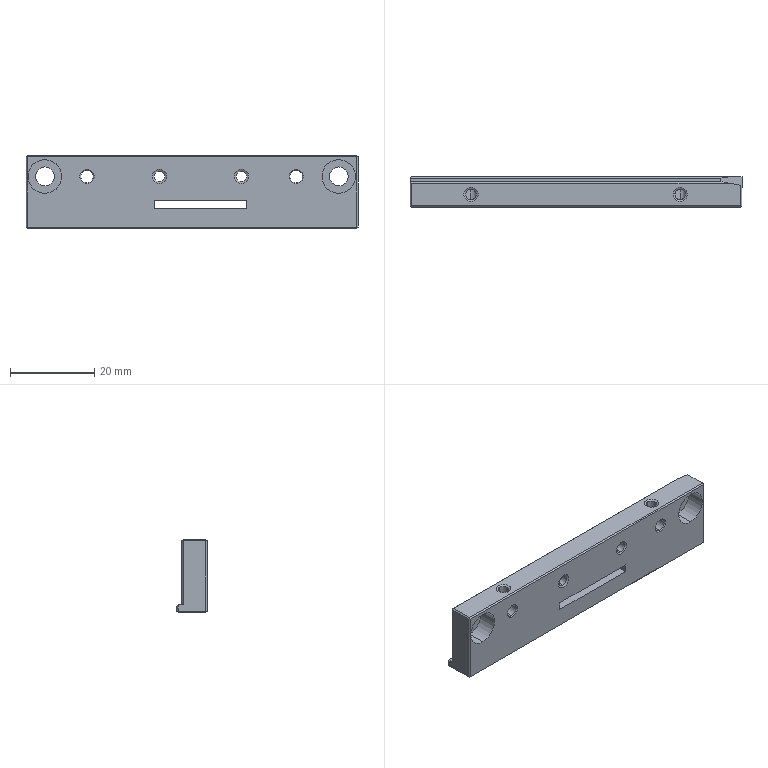Part | NX | 1 solid | 62 faces | box 79 x 7.2 x 17.4 mm | volume 7427 mm3 | plane 30 | cylinder 20 | cone 12 | commonest cylinder face diameters 2.5 x8 3 x4 4.5 x4 8 x4